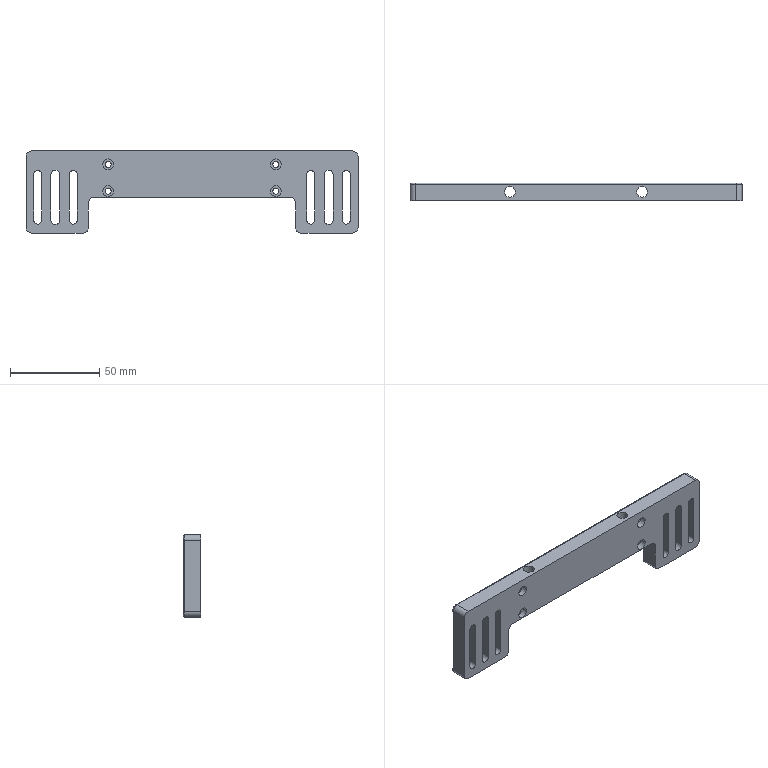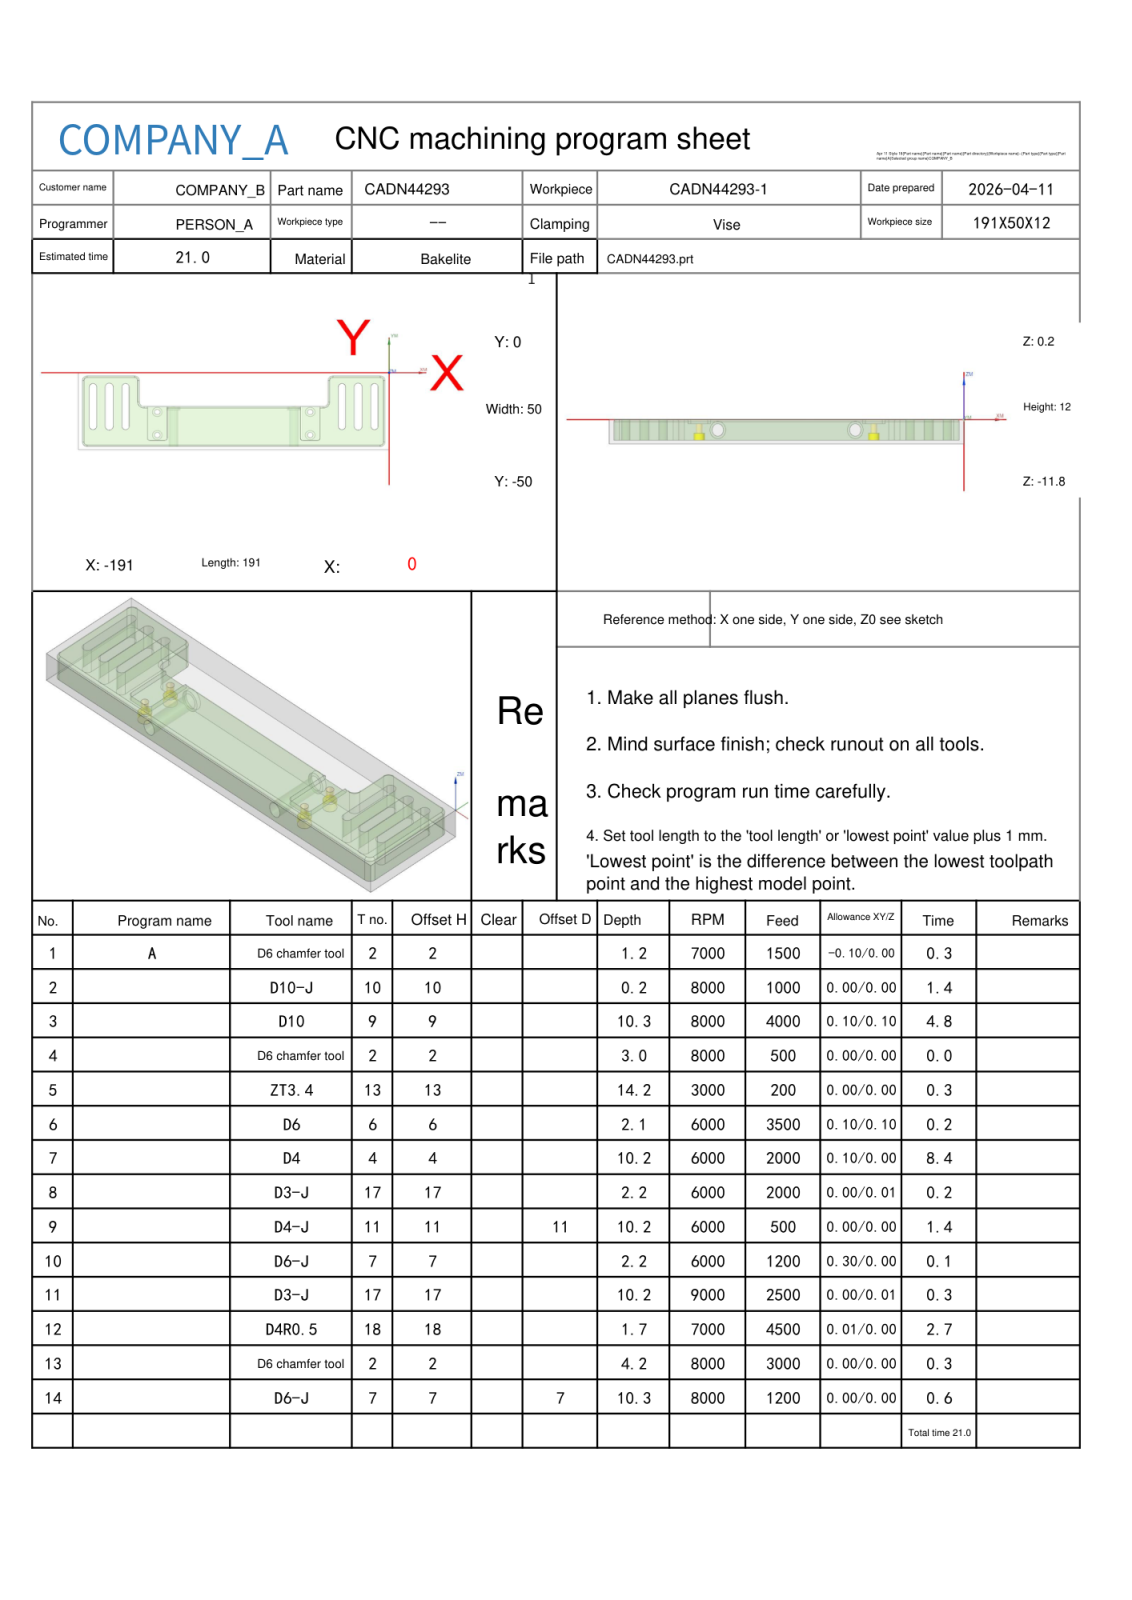NC program | NX | posted by the shop | part box 186 x 10 x 46 mm
Lines 4734 to 6466 of 7485, first 1444 of 1733 lines:
N11 T17 M06
(D3-J  D=3. R=0. H=17 ce=0.00 di=0.01)
G00 G90 G54 X-151.968 Y-16.863 M03 S9000
G43 H17 Z20.
M08
Z.474
G01 X-151.972 Y-16.864 Z.401 F2000.
X-151.984 Y-16.866 Z.328
X-152.001 Y-16.871 Z.256
X-152.024 Y-16.878 Z.185
X-152.051 Y-16.887 Z.115
X-152.081 Y-16.899 Z.049
X-152.112 Y-16.914 Z-.014
X-152.144 Y-16.932 Z-.073
X-152.176 Y-16.954 Z-.127
X-152.205 Y-16.978 Z-.174
X-152.232 Y-17.007 Z-.215
X-152.255 Y-17.04 Z-.247
X-152.273 Y-17.076 Z-.272
X-152.284 Y-17.117 Z-.287
X-152.288 Y-17.163 Z-.293
Y-19. F2500.
G03 X-150.5 Y-20.788 I1.788 J0.0
G01 X-148.663
X-148.634 Y-20.773 Z-.29
X-148.627 Y-20.729 Z-.283
X-148.642 Y-20.659 Z-.273
X-148.675 Y-20.567 Z-.26
X-148.726 Y-20.454 Z-.245
X-148.792 Y-20.324 Z-.23
X-148.964 Y-20.028 Z-.201
X-149.086 Y-19.835 Z-.186
X-149.298 Y-19.518 Z-.17
X-149.578 Y-19.138
X-149.88 Y-18.764 Z-.188
X-150.2 Y-18.401 Z-.223
X-150.535 Y-18.055 Z-.271
X-150.882 Y-17.731 Z-.331
X-151.178 Y-17.483 Z-.389
X-151.36 Y-17.341 Z-.426
X-151.641 Y-17.138 Z-.485
X-151.765 Y-17.059 Z-.512
X-151.873 Y-16.996 Z-.536
X-151.963 Y-16.954 Z-.557
X-152.03 Y-16.933 Z-.572
X-152.073 Y-16.935 Z-.582
X-152.088 Y-16.962 Z-.585
Y-19.
G03 X-150.5 Y-20.588 I1.588 J0.0
G01 X-148.55
X-148.521 Y-20.572 Z-.584
X-148.514 Y-20.527 Z-.582
X-148.529 Y-20.456 Z-.578
X-148.562 Y-20.361 Z-.574
X-148.612 Y-20.246 Z-.57
X-148.679 Y-20.115 Z-.565
X-148.85 Y-19.816 Z-.56
X-148.971 Y-19.622 Z-.558
X-149.183 Y-19.307 Z-.562
X-149.536 Y-18.844 Z-.583
X-149.923 Y-18.399 Z-.62
X-150.338 Y-17.98 Z-.668
X-150.774 Y-17.595 Z-.723
X-151.075 Y-17.363 Z-.761
X-151.261 Y-17.229 Z-.785
X-151.548 Y-17.04 Z-.821
X-151.675 Y-16.966 Z-.837
X-151.787 Y-16.909 Z-.85
X-151.878 Y-16.871 Z-.862
X-151.948 Y-16.852 Z-.871
X-151.992 Y-16.857 Z-.876
X-152.007 Y-16.885 Z-.878
Y-19.
G03 X-150.5 Y-20.507 I1.507 J0.0
G01 X-148.55
X-148.521 Y-20.491
X-148.514 Y-20.446 Z-.88
X-148.528 Y-20.374 Z-.882
X-148.561 Y-20.279 Z-.885
X-148.612 Y-20.164 Z-.889
X-148.678 Y-20.032 Z-.893
X-148.848 Y-19.734 Z-.906
X-148.969 Y-19.541 Z-.915
X-149.181 Y-19.228 Z-.932
X-149.532 Y-18.771 Z-.963
X-149.918 Y-18.336 Z-.999
X-150.332 Y-17.929 Z-1.038
X-150.768 Y-17.556 Z-1.077
X-151.068 Y-17.331 Z-1.102
X-151.254 Y-17.203 Z-1.116
X-151.541 Y-17.02 Z-1.138
X-151.669 Y-16.949 Z-1.147
X-151.78 Y-16.895 Z-1.155
X-151.871 Y-16.858 Z-1.162
X-151.941 Y-16.842 Z-1.167
X-151.985 Y-16.847 Z-1.17
X-152. Y-16.875 Z-1.171
Y-19.
G03 X-150.5 Y-20.5 I1.5 J0.0
G01 X-148.55
X-148.521 Y-20.484
X-148.514 Y-20.439 Z-1.174
X-148.528 Y-20.367 Z-1.178
X-148.561 Y-20.272 Z-1.184
X-148.612 Y-20.157 Z-1.19
X-148.678 Y-20.025 Z-1.198
X-148.848 Y-19.728 Z-1.217
X-148.969 Y-19.534 Z-1.229
X-149.181 Y-19.221 Z-1.25
X-149.532 Y-18.766 Z-1.283
X-149.918 Y-18.331 Z-1.317
X-150.332 Y-17.925 Z-1.351
X-150.768 Y-17.554 Z-1.384
X-151.068 Y-17.329 Z-1.405
X-151.254 Y-17.201 Z-1.417
X-151.541 Y-17.019 Z-1.436
X-151.669 Y-16.949 Z-1.443
X-151.78 Y-16.894 Z-1.45
X-151.871 Y-16.858 Z-1.456
X-151.941 Y-16.841 Z-1.46
X-151.985 Y-16.847 Z-1.462
X-152. Y-16.875 Z-1.463
Y-19.
G03 X-150.5 Y-20.5 I1.5 J0.0
G01 X-148.55
X-148.521 Y-20.484 Z-1.464
X-148.514 Y-20.439 Z-1.467
X-148.528 Y-20.367 Z-1.471
X-148.561 Y-20.272 Z-1.476
X-148.612 Y-20.157 Z-1.483
X-148.678 Y-20.025 Z-1.491
X-148.848 Y-19.728 Z-1.509
X-148.969 Y-19.534 Z-1.522
X-149.181 Y-19.221 Z-1.542
X-149.532 Y-18.766 Z-1.575
X-149.918 Y-18.331 Z-1.61
X-150.332 Y-17.925 Z-1.644
X-150.768 Y-17.554 Z-1.677
X-151.068 Y-17.329 Z-1.697
X-151.254 Y-17.201 Z-1.71
X-151.541 Y-17.019 Z-1.728
X-151.669 Y-16.949 Z-1.736
X-151.78 Y-16.894 Z-1.743
X-151.871 Y-16.858 Z-1.748
X-151.941 Y-16.841 Z-1.752
X-151.985 Y-16.846 Z-1.755
X-152. Y-16.875 Z-1.756
Y-19.
G03 X-150.5 Y-20.5 I1.5 J0.0
G01 X-148.55
X-148.521 Y-20.484 Z-1.757
X-148.514 Y-20.439 Z-1.759
X-148.528 Y-20.367 Z-1.763
X-148.561 Y-20.272 Z-1.769
X-148.612 Y-20.157 Z-1.776
X-148.678 Y-20.025 Z-1.784
X-148.848 Y-19.728 Z-1.802
X-148.969 Y-19.534 Z-1.814
X-149.181 Y-19.221 Z-1.835
X-149.532 Y-18.765 Z-1.868
X-149.918 Y-18.331 Z-1.902
X-150.332 Y-17.925 Z-1.936
X-150.768 Y-17.553 Z-1.969
X-151.068 Y-17.329 Z-1.99
X-151.254 Y-17.201 Z-2.002
X-151.541 Y-17.019 Z-2.021
X-151.669 Y-16.948 Z-2.029
X-151.78 Y-16.894 Z-2.035
X-151.871 Y-16.858 Z-2.041
X-151.941 Y-16.841 Z-2.045
X-151.985 Y-16.846 Z-2.048
X-152. Y-16.875 Z-2.049
Y-19.
G03 X-150.5 Y-20.5 I1.5 J0.0
G01 X-148.375
X-148.346 Y-20.484
X-148.341 Y-20.439 Z-2.052
X-148.357 Y-20.367 Z-2.056
X-148.394 Y-20.272 Z-2.062
X-148.448 Y-20.157 Z-2.068
X-148.519 Y-20.025 Z-2.076
X-148.7 Y-19.727 Z-2.095
X-148.829 Y-19.534 Z-2.107
X-149.053 Y-19.221 Z-2.128
X-149.424 Y-18.765 Z-2.161
X-149.83 Y-18.331 Z-2.195
X-150.265 Y-17.925 Z-2.229
X-150.72 Y-17.553 Z-2.262
X-151.034 Y-17.329 Z-2.283
X-151.227 Y-17.201 Z-2.295
X-151.525 Y-17.019 Z-2.313
X-151.657 Y-16.948 Z-2.321
X-151.772 Y-16.894 Z-2.328
X-151.867 Y-16.858 Z-2.334
X-151.939 Y-16.841 Z-2.338
X-151.984 Y-16.846 Z-2.34
X-152. Y-16.875 Z-2.341
Y-19.
G03 X-150.5 Y-20.5 I1.5 J0.0
G01 X-148.375
X-148.346 Y-20.484 Z-2.342
X-148.341 Y-20.439 Z-2.345
X-148.357 Y-20.367 Z-2.349
X-148.394 Y-20.272 Z-2.354
X-148.448 Y-20.157 Z-2.361
X-148.519 Y-20.025 Z-2.369
X-148.7 Y-19.727 Z-2.387
X-148.829 Y-19.534 Z-2.4
X-149.053 Y-19.221 Z-2.42
X-149.424 Y-18.765 Z-2.453
X-149.83 Y-18.331 Z-2.488
X-150.265 Y-17.925 Z-2.522
X-150.72 Y-17.553 Z-2.555
X-151.034 Y-17.329 Z-2.575
X-151.227 Y-17.201 Z-2.588
X-151.525 Y-17.019 Z-2.606
X-151.657 Y-16.948 Z-2.614
X-151.772 Y-16.894 Z-2.621
X-151.867 Y-16.858 Z-2.626
X-151.939 Y-16.841 Z-2.63
X-151.984 Y-16.846 Z-2.633
X-152. Y-16.875 Z-2.634
Y-19.
G03 X-150.5 Y-20.5 I1.5 J0.0
G01 X-148.375
X-148.346 Y-20.484 Z-2.635
X-148.341 Y-20.439 Z-2.637
X-148.357 Y-20.367 Z-2.641
X-148.394 Y-20.272 Z-2.647
X-148.448 Y-20.157 Z-2.654
X-148.519 Y-20.025 Z-2.662
X-148.7 Y-19.727 Z-2.68
X-148.829 Y-19.534 Z-2.692
X-149.053 Y-19.221 Z-2.713
X-149.424 Y-18.765 Z-2.746
X-149.83 Y-18.331 Z-2.78
X-150.265 Y-17.925 Z-2.814
X-150.72 Y-17.553 Z-2.847
X-151.034 Y-17.329 Z-2.868
X-151.227 Y-17.201 Z-2.88
X-151.525 Y-17.019 Z-2.899
X-151.657 Y-16.948 Z-2.907
X-151.772 Y-16.894 Z-2.913
X-151.867 Y-16.858 Z-2.919
X-151.939 Y-16.841 Z-2.923
X-151.984 Y-16.846 Z-2.926
X-152. Y-16.875
Y-19.
G03 X-150.5 Y-20.5 I1.5 J0.0
G01 X-148.375
X-148.346 Y-20.484 Z-2.927
X-148.341 Y-20.439 Z-2.93
X-148.357 Y-20.367 Z-2.934
X-148.394 Y-20.272 Z-2.94
X-148.448 Y-20.157 Z-2.946
X-148.519 Y-20.025 Z-2.954
X-148.7 Y-19.727 Z-2.973
X-148.829 Y-19.534 Z-2.985
X-149.053 Y-19.221 Z-3.006
X-149.424 Y-18.765 Z-3.039
X-149.83 Y-18.331 Z-3.073
X-150.265 Y-17.925 Z-3.107
X-150.72 Y-17.553 Z-3.14
X-151.034 Y-17.329 Z-3.161
X-151.227 Y-17.201 Z-3.173
X-151.525 Y-17.019 Z-3.191
X-151.657 Y-16.948 Z-3.199
X-151.772 Y-16.894 Z-3.206
X-151.867 Y-16.858 Z-3.212
X-151.939 Y-16.841 Z-3.216
X-151.984 Y-16.846 Z-3.218
X-152. Y-16.875 Z-3.219
Y-19.
G03 X-150.5 Y-20.5 I1.5 J0.0
G01 X-148.375
X-148.346 Y-20.484 Z-3.22
X-148.341 Y-20.439 Z-3.223
X-148.357 Y-20.367 Z-3.227
X-148.394 Y-20.272 Z-3.232
X-148.448 Y-20.157 Z-3.239
X-148.519 Y-20.025 Z-3.247
X-148.7 Y-19.727 Z-3.265
X-148.829 Y-19.534 Z-3.278
X-149.053 Y-19.221 Z-3.298
X-149.424 Y-18.765 Z-3.331
X-149.83 Y-18.331 Z-3.365
X-150.265 Y-17.925 Z-3.4
X-150.72 Y-17.553 Z-3.433
X-151.034 Y-17.329 Z-3.453
X-151.227 Y-17.201 Z-3.466
X-151.525 Y-17.019 Z-3.484
X-151.657 Y-16.948 Z-3.492
X-151.772 Y-16.894 Z-3.499
X-151.867 Y-16.858 Z-3.504
X-151.939 Y-16.841 Z-3.508
X-151.984 Y-16.846 Z-3.511
X-152. Y-16.875 Z-3.512
Y-19.
G03 X-150.5 Y-20.5 I1.5 J0.0
G01 X-148.375
X-148.346 Y-20.484 Z-3.513
X-148.341 Y-20.439 Z-3.515
X-148.357 Y-20.367 Z-3.519
X-148.394 Y-20.272 Z-3.525
X-148.448 Y-20.157 Z-3.532
X-148.519 Y-20.025 Z-3.539
X-148.7 Y-19.727 Z-3.558
X-148.829 Y-19.534 Z-3.57
X-149.053 Y-19.221 Z-3.591
X-149.424 Y-18.765 Z-3.624
X-149.83 Y-18.331 Z-3.658
X-150.265 Y-17.925 Z-3.692
X-150.72 Y-17.553 Z-3.725
X-151.034 Y-17.329 Z-3.746
X-151.227 Y-17.201 Z-3.758
X-151.525 Y-17.019 Z-3.777
X-151.657 Y-16.948 Z-3.785
X-151.772 Y-16.894 Z-3.791
X-151.867 Y-16.858 Z-3.797
X-151.939 Y-16.841 Z-3.801
X-151.984 Y-16.846 Z-3.804
X-152. Y-16.875
Y-19.
G03 X-150.5 Y-20.5 I1.5 J0.0
G01 X-148.375
X-148.346 Y-20.484 Z-3.805
X-148.341 Y-20.439 Z-3.808
X-148.357 Y-20.367 Z-3.812
X-148.394 Y-20.272 Z-3.817
X-148.448 Y-20.157 Z-3.824
X-148.519 Y-20.025 Z-3.832
X-148.7 Y-19.727 Z-3.85
X-148.829 Y-19.534 Z-3.863
X-149.053 Y-19.221 Z-3.884
X-149.424 Y-18.765 Z-3.917
X-149.83 Y-18.331 Z-3.951
X-150.265 Y-17.925 Z-3.985
X-150.72 Y-17.553 Z-4.018
X-151.034 Y-17.329 Z-4.039
X-151.227 Y-17.201 Z-4.051
X-151.525 Y-17.019 Z-4.069
X-151.657 Y-16.948 Z-4.077
X-151.772 Y-16.894 Z-4.084
X-151.867 Y-16.858 Z-4.09
X-151.939 Y-16.841 Z-4.094
X-151.984 Y-16.846 Z-4.096
X-152. Y-16.875 Z-4.097
Y-19.
G03 X-150.5 Y-20.5 I1.5 J0.0
G01 X-148.375
X-148.346 Y-20.484 Z-4.098
X-148.341 Y-20.439 Z-4.101
X-148.357 Y-20.367 Z-4.105
X-148.394 Y-20.272 Z-4.11
X-148.448 Y-20.157 Z-4.117
X-148.519 Y-20.025 Z-4.125
X-148.7 Y-19.727 Z-4.143
X-148.829 Y-19.534 Z-4.155
X-149.053 Y-19.221 Z-4.176
X-149.424 Y-18.765 Z-4.209
X-149.83 Y-18.331 Z-4.243
X-150.265 Y-17.925 Z-4.277
X-150.72 Y-17.553 Z-4.31
X-151.034 Y-17.329 Z-4.331
X-151.227 Y-17.201 Z-4.344
X-151.525 Y-17.019 Z-4.362
X-151.657 Y-16.948 Z-4.37
X-151.772 Y-16.894 Z-4.377
X-151.867 Y-16.858 Z-4.382
X-151.939 Y-16.841 Z-4.386
X-151.984 Y-16.846 Z-4.389
X-152. Y-16.875 Z-4.39
Y-19.
G03 X-150.5 Y-20.5 I1.5 J0.0
G01 X-148.375
X-148.346 Y-20.484 Z-4.391
X-148.341 Y-20.439 Z-4.393
X-148.357 Y-20.367 Z-4.397
X-148.394 Y-20.272 Z-4.403
X-148.448 Y-20.157 Z-4.41
X-148.519 Y-20.025 Z-4.417
X-148.7 Y-19.727 Z-4.436
X-148.829 Y-19.534 Z-4.448
X-149.053 Y-19.221 Z-4.469
X-149.424 Y-18.765 Z-4.502
X-149.83 Y-18.331 Z-4.536
X-150.265 Y-17.925 Z-4.57
X-150.72 Y-17.553 Z-4.603
X-151.034 Y-17.329 Z-4.624
X-151.227 Y-17.201 Z-4.636
X-151.525 Y-17.019 Z-4.655
X-151.657 Y-16.948 Z-4.663
X-151.772 Y-16.894 Z-4.669
X-151.867 Y-16.858 Z-4.675
X-151.939 Y-16.841 Z-4.679
X-151.984 Y-16.846 Z-4.681
X-152. Y-16.875 Z-4.682
Y-19.
G03 X-150.5 Y-20.5 I1.5 J0.0
G01 X-148.375
X-148.346 Y-20.484 Z-4.683
X-148.341 Y-20.439 Z-4.686
X-148.357 Y-20.367 Z-4.69
X-148.394 Y-20.272 Z-4.695
X-148.448 Y-20.157 Z-4.702
X-148.519 Y-20.025 Z-4.71
X-148.7 Y-19.727 Z-4.728
X-148.829 Y-19.534 Z-4.741
X-149.053 Y-19.221 Z-4.762
X-149.424 Y-18.765 Z-4.795
X-149.83 Y-18.331 Z-4.829
X-150.265 Y-17.925 Z-4.863
X-150.72 Y-17.553 Z-4.896
X-151.034 Y-17.329 Z-4.917
X-151.227 Y-17.201 Z-4.929
X-151.525 Y-17.019 Z-4.947
X-151.657 Y-16.948 Z-4.955
X-151.772 Y-16.894 Z-4.962
X-151.867 Y-16.858 Z-4.967
X-151.939 Y-16.841 Z-4.972
X-151.984 Y-16.846 Z-4.974
X-152. Y-16.875 Z-4.975
Y-19.
G03 X-150.5 Y-20.5 I1.5 J0.0
G01 X-148.375
X-148.346 Y-20.484 Z-4.976
X-148.341 Y-20.439 Z-4.978
X-148.357 Y-20.367 Z-4.983
X-148.394 Y-20.272 Z-4.988
X-148.448 Y-20.157 Z-4.995
X-148.519 Y-20.025 Z-5.003
X-148.7 Y-19.727 Z-5.021
X-148.829 Y-19.534 Z-5.033
X-149.053 Y-19.221 Z-5.054
X-149.424 Y-18.765 Z-5.087
X-149.83 Y-18.331 Z-5.121
X-150.265 Y-17.925 Z-5.155
X-150.72 Y-17.553 Z-5.188
X-151.034 Y-17.329 Z-5.209
X-151.227 Y-17.201 Z-5.222
X-151.525 Y-17.019 Z-5.24
X-151.657 Y-16.948 Z-5.248
X-151.772 Y-16.894 Z-5.255
X-151.867 Y-16.858 Z-5.26
X-151.939 Y-16.841 Z-5.264
X-151.984 Y-16.846 Z-5.267
X-152. Y-16.875 Z-5.268
Y-19.
G03 X-150.5 Y-20.5 I1.5 J0.0
G01 X-148.375
X-148.346 Y-20.484 Z-5.269
X-148.341 Y-20.439 Z-5.271
X-148.357 Y-20.367 Z-5.275
X-148.394 Y-20.272 Z-5.281
X-148.448 Y-20.157 Z-5.287
X-148.519 Y-20.025 Z-5.295
X-148.7 Y-19.727 Z-5.314
X-148.829 Y-19.534 Z-5.326
X-149.053 Y-19.221 Z-5.347
X-149.424 Y-18.765 Z-5.38
X-149.83 Y-18.331 Z-5.414
X-150.265 Y-17.925 Z-5.448
X-150.72 Y-17.553 Z-5.481
X-151.034 Y-17.329 Z-5.502
X-151.227 Y-17.201 Z-5.514
X-151.525 Y-17.019 Z-5.533
X-151.657 Y-16.948 Z-5.54
X-151.772 Y-16.894 Z-5.547
X-151.867 Y-16.858 Z-5.553
X-151.939 Y-16.841 Z-5.557
X-151.984 Y-16.846 Z-5.559
X-152. Y-16.875 Z-5.56
Y-19.
G03 X-150.5 Y-20.5 I1.5 J0.0
G01 X-148.375
X-148.346 Y-20.484 Z-5.561
X-148.341 Y-20.439 Z-5.564
X-148.357 Y-20.367 Z-5.568
X-148.394 Y-20.272 Z-5.573
X-148.448 Y-20.157 Z-5.58
X-148.519 Y-20.025 Z-5.588
X-148.7 Y-19.727 Z-5.606
X-148.829 Y-19.534 Z-5.619
X-149.053 Y-19.221 Z-5.64
X-149.424 Y-18.765 Z-5.673
X-149.83 Y-18.331 Z-5.707
X-150.265 Y-17.925 Z-5.741
X-150.72 Y-17.553 Z-5.774
X-151.034 Y-17.329 Z-5.795
X-151.227 Y-17.201 Z-5.807
X-151.525 Y-17.019 Z-5.825
X-151.657 Y-16.948 Z-5.833
X-151.772 Y-16.894 Z-5.84
X-151.867 Y-16.858 Z-5.845
X-151.939 Y-16.841 Z-5.849
X-151.984 Y-16.846 Z-5.852
X-152. Y-16.875 Z-5.853
Y-19.
G03 X-150.5 Y-20.5 I1.5 J0.0
G01 X-148.375
X-148.346 Y-20.484 Z-5.854
X-148.341 Y-20.439 Z-5.856
X-148.357 Y-20.367 Z-5.86
X-148.394 Y-20.272 Z-5.866
X-148.448 Y-20.157 Z-5.873
X-148.519 Y-20.025 Z-5.881
X-148.7 Y-19.727 Z-5.899
X-148.829 Y-19.534 Z-5.911
X-149.053 Y-19.221 Z-5.932
X-149.424 Y-18.765 Z-5.965
X-149.83 Y-18.331 Z-5.999
X-150.265 Y-17.925 Z-6.033
X-150.72 Y-17.553 Z-6.066
X-151.034 Y-17.329 Z-6.087
X-151.227 Y-17.201 Z-6.1
X-151.525 Y-17.019 Z-6.118
X-151.657 Y-16.948 Z-6.126
X-151.772 Y-16.894 Z-6.133
X-151.867 Y-16.858 Z-6.138
X-151.939 Y-16.841 Z-6.142
X-151.984 Y-16.846 Z-6.145
X-152. Y-16.875 Z-6.146
Y-19.
G03 X-150.5 Y-20.5 I1.5 J0.0
G01 X-148.375
X-148.346 Y-20.484
X-148.341 Y-20.439 Z-6.149
X-148.357 Y-20.367 Z-6.153
X-148.394 Y-20.272 Z-6.159
X-148.448 Y-20.157 Z-6.165
X-148.519 Y-20.025 Z-6.173
X-148.7 Y-19.727 Z-6.192
X-148.829 Y-19.534 Z-6.204
X-149.053 Y-19.221 Z-6.225
X-149.424 Y-18.765 Z-6.258
X-149.83 Y-18.331 Z-6.292
X-150.265 Y-17.925 Z-6.326
X-150.72 Y-17.553 Z-6.359
X-151.034 Y-17.329 Z-6.38
X-151.227 Y-17.201 Z-6.392
X-151.525 Y-17.019 Z-6.411
X-151.657 Y-16.948 Z-6.418
X-151.772 Y-16.894 Z-6.425
X-151.867 Y-16.858 Z-6.431
X-151.939 Y-16.841 Z-6.435
X-151.984 Y-16.846 Z-6.437
X-152. Y-16.875 Z-6.438
Y-19.
G03 X-150.5 Y-20.5 I1.5 J0.0
G01 X-148.375
X-148.346 Y-20.484 Z-6.439
X-148.341 Y-20.439 Z-6.442
X-148.357 Y-20.367 Z-6.446
X-148.394 Y-20.272 Z-6.451
X-148.448 Y-20.157 Z-6.458
X-148.519 Y-20.025 Z-6.466
X-148.7 Y-19.727 Z-6.484
X-148.829 Y-19.534 Z-6.497
X-149.053 Y-19.221 Z-6.517
X-149.424 Y-18.765 Z-6.55
X-149.83 Y-18.331 Z-6.585
X-150.265 Y-17.925 Z-6.619
X-150.72 Y-17.553 Z-6.652
X-151.034 Y-17.329 Z-6.672
X-151.227 Y-17.201 Z-6.685
X-151.525 Y-17.019 Z-6.703
X-151.657 Y-16.948 Z-6.711
X-151.772 Y-16.894 Z-6.718
X-151.867 Y-16.858 Z-6.723
X-151.939 Y-16.841 Z-6.727
X-151.984 Y-16.846 Z-6.73
X-152. Y-16.875 Z-6.731
Y-19.
G03 X-150.5 Y-20.5 I1.5 J0.0
G01 X-148.375
X-148.346 Y-20.484 Z-6.732
X-148.341 Y-20.439 Z-6.734
X-148.357 Y-20.367 Z-6.738
X-148.394 Y-20.272 Z-6.744
X-148.448 Y-20.157 Z-6.751
X-148.519 Y-20.025 Z-6.759
X-148.7 Y-19.727 Z-6.777
X-148.829 Y-19.534 Z-6.789
X-149.053 Y-19.221 Z-6.81
X-149.424 Y-18.765 Z-6.843
X-149.83 Y-18.331 Z-6.877
X-150.265 Y-17.925 Z-6.911
X-150.72 Y-17.553 Z-6.944
X-151.034 Y-17.329 Z-6.965
X-151.227 Y-17.201 Z-6.977
X-151.525 Y-17.019 Z-6.996
X-151.657 Y-16.948 Z-7.004
X-151.772 Y-16.894 Z-7.01
X-151.867 Y-16.858 Z-7.016
X-151.939 Y-16.841 Z-7.02
X-151.984 Y-16.846 Z-7.023
X-152. Y-16.875 Z-7.024
Y-19.
G03 X-150.5 Y-20.5 I1.5 J0.0
G01 X-148.375
X-148.346 Y-20.484
X-148.341 Y-20.439 Z-7.027
X-148.357 Y-20.367 Z-7.031
X-148.394 Y-20.272 Z-7.037
X-148.448 Y-20.157 Z-7.043
X-148.519 Y-20.025 Z-7.051
X-148.7 Y-19.727 Z-7.07
X-148.829 Y-19.534 Z-7.082
X-149.053 Y-19.221 Z-7.103
X-149.424 Y-18.765 Z-7.136
X-149.83 Y-18.331 Z-7.17
X-150.265 Y-17.925 Z-7.204
X-150.72 Y-17.553 Z-7.237
X-151.034 Y-17.329 Z-7.258
X-151.227 Y-17.201 Z-7.27
X-151.525 Y-17.019 Z-7.288
X-151.657 Y-16.948 Z-7.296
X-151.772 Y-16.894 Z-7.303
X-151.867 Y-16.858 Z-7.309
X-151.939 Y-16.841 Z-7.313
X-151.984 Y-16.846 Z-7.315
X-152. Y-16.875 Z-7.316
Y-19.
G03 X-150.5 Y-20.5 I1.5 J0.0
G01 X-148.375
X-148.346 Y-20.484 Z-7.317
X-148.341 Y-20.439 Z-7.32
X-148.357 Y-20.367 Z-7.324
X-148.394 Y-20.272 Z-7.329
X-148.448 Y-20.157 Z-7.336
X-148.519 Y-20.025 Z-7.344
X-148.7 Y-19.727 Z-7.362
X-148.829 Y-19.534 Z-7.375
X-149.053 Y-19.221 Z-7.395
X-149.424 Y-18.765 Z-7.428
X-149.83 Y-18.331 Z-7.463
X-150.265 Y-17.925 Z-7.497
X-150.72 Y-17.553 Z-7.53
X-151.034 Y-17.329 Z-7.55
X-151.227 Y-17.201 Z-7.563
X-151.525 Y-17.019 Z-7.581
X-151.657 Y-16.948 Z-7.589
X-151.772 Y-16.894 Z-7.596
X-151.867 Y-16.858 Z-7.601
X-151.939 Y-16.841 Z-7.605
X-151.984 Y-16.846 Z-7.608
X-152. Y-16.875 Z-7.609
Y-19.
G03 X-150.5 Y-20.5 I1.5 J0.0
G01 X-148.375
X-148.346 Y-20.484 Z-7.61
X-148.341 Y-20.439 Z-7.612
X-148.357 Y-20.367 Z-7.616
X-148.394 Y-20.272 Z-7.622
X-148.448 Y-20.157 Z-7.629
X-148.519 Y-20.025 Z-7.637
X-148.7 Y-19.727 Z-7.655
X-148.829 Y-19.534 Z-7.667
X-149.053 Y-19.221 Z-7.688
X-149.424 Y-18.765 Z-7.721
X-149.83 Y-18.331 Z-7.755
X-150.265 Y-17.925 Z-7.789
X-150.72 Y-17.553 Z-7.822
X-151.034 Y-17.329 Z-7.843
X-151.227 Y-17.201 Z-7.855
X-151.525 Y-17.019 Z-7.874
X-151.657 Y-16.948 Z-7.882
X-151.772 Y-16.894 Z-7.888
X-151.867 Y-16.858 Z-7.894
X-151.939 Y-16.841 Z-7.898
X-151.984 Y-16.846 Z-7.901
X-152. Y-16.875
Y-19.
G03 X-150.5 Y-20.5 I1.5 J0.0
G01 X-148.375
X-148.346 Y-20.484 Z-7.902
X-148.341 Y-20.439 Z-7.905
X-148.357 Y-20.367 Z-7.909
X-148.394 Y-20.272 Z-7.915
X-148.448 Y-20.157 Z-7.921
X-148.519 Y-20.025 Z-7.929
X-148.7 Y-19.727 Z-7.948
X-148.829 Y-19.534 Z-7.96
X-149.053 Y-19.221 Z-7.981
X-149.424 Y-18.765 Z-8.014
X-149.83 Y-18.331 Z-8.048
X-150.265 Y-17.925 Z-8.082
X-150.72 Y-17.553 Z-8.115
X-151.034 Y-17.329 Z-8.136
X-151.227 Y-17.201 Z-8.148
X-151.525 Y-17.019 Z-8.166
X-151.657 Y-16.948 Z-8.174
X-151.772 Y-16.894 Z-8.181
X-151.867 Y-16.858 Z-8.187
X-151.939 Y-16.841 Z-8.191
X-151.984 Y-16.846 Z-8.193
X-152. Y-16.875 Z-8.194
Y-19.
G03 X-150.5 Y-20.5 I1.5 J0.0
G01 X-148.375
X-148.346 Y-20.484 Z-8.195
X-148.341 Y-20.439 Z-8.198
X-148.357 Y-20.367 Z-8.202
X-148.394 Y-20.272 Z-8.207
X-148.448 Y-20.157 Z-8.214
X-148.519 Y-20.025 Z-8.222
X-148.7 Y-19.727 Z-8.24
X-148.829 Y-19.534 Z-8.253
X-149.053 Y-19.221 Z-8.273
X-149.424 Y-18.765 Z-8.306
X-149.83 Y-18.331 Z-8.34
X-150.265 Y-17.925 Z-8.375
X-150.72 Y-17.553 Z-8.408
X-151.034 Y-17.329 Z-8.428
X-151.227 Y-17.201 Z-8.441
X-151.525 Y-17.019 Z-8.459
X-151.657 Y-16.948 Z-8.467
X-151.772 Y-16.894 Z-8.474
X-151.867 Y-16.858 Z-8.479
X-151.939 Y-16.841 Z-8.483
X-151.984 Y-16.846 Z-8.486
X-152. Y-16.875 Z-8.487
Y-19.
G03 X-150.5 Y-20.5 I1.5 J0.0
G01 X-148.375
X-148.346 Y-20.484 Z-8.488
X-148.341 Y-20.439 Z-8.49
X-148.357 Y-20.367 Z-8.494
X-148.394 Y-20.272 Z-8.5
X-148.448 Y-20.157 Z-8.507
X-148.519 Y-20.025 Z-8.514
X-148.7 Y-19.727 Z-8.533
X-148.829 Y-19.534 Z-8.545
X-149.053 Y-19.221 Z-8.566
X-149.424 Y-18.765 Z-8.599
X-149.83 Y-18.331 Z-8.633
X-150.265 Y-17.925 Z-8.667
X-150.72 Y-17.553 Z-8.7
X-151.034 Y-17.329 Z-8.721
X-151.227 Y-17.201 Z-8.733
X-151.525 Y-17.019 Z-8.752
X-151.657 Y-16.948 Z-8.76
X-151.772 Y-16.894 Z-8.766
X-151.867 Y-16.858 Z-8.772
X-151.939 Y-16.841 Z-8.776
X-151.984 Y-16.846 Z-8.779
X-152. Y-16.875
Y-19.
G03 X-150.5 Y-20.5 I1.5 J0.0
G01 X-148.375
X-148.346 Y-20.484 Z-8.78
X-148.341 Y-20.439 Z-8.783
X-148.357 Y-20.367 Z-8.787
X-148.394 Y-20.272 Z-8.792
X-148.448 Y-20.157 Z-8.799
X-148.519 Y-20.025 Z-8.807
X-148.7 Y-19.727 Z-8.825
X-148.829 Y-19.534 Z-8.838
X-149.053 Y-19.221 Z-8.859
X-149.424 Y-18.765 Z-8.892
X-149.83 Y-18.331 Z-8.926
X-150.265 Y-17.925 Z-8.96
X-150.72 Y-17.553 Z-8.993
X-151.034 Y-17.329 Z-9.014
X-151.227 Y-17.201 Z-9.026
X-151.525 Y-17.019 Z-9.044
X-151.657 Y-16.948 Z-9.052
X-151.772 Y-16.894 Z-9.059
X-151.867 Y-16.858 Z-9.065
X-151.939 Y-16.841 Z-9.069
X-151.984 Y-16.846 Z-9.071
X-152. Y-16.875 Z-9.072
Y-19.
G03 X-150.5 Y-20.5 I1.5 J0.0
G01 X-148.375
X-148.346 Y-20.484 Z-9.073
X-148.341 Y-20.439 Z-9.076
X-148.357 Y-20.367 Z-9.08
X-148.394 Y-20.272 Z-9.085
X-148.448 Y-20.157 Z-9.092
X-148.519 Y-20.025 Z-9.1
X-148.7 Y-19.727 Z-9.118
X-148.829 Y-19.534 Z-9.13
X-149.053 Y-19.221 Z-9.151
X-149.424 Y-18.765 Z-9.184
X-149.83 Y-18.331 Z-9.218
X-150.265 Y-17.925 Z-9.252
X-150.72 Y-17.553 Z-9.285
X-151.034 Y-17.329 Z-9.306
X-151.227 Y-17.201 Z-9.319
X-151.525 Y-17.019 Z-9.337
X-151.657 Y-16.948 Z-9.345
X-151.772 Y-16.894 Z-9.352
X-151.867 Y-16.858 Z-9.357
X-151.939 Y-16.841 Z-9.361
X-151.984 Y-16.846 Z-9.364
X-152. Y-16.875 Z-9.365
Y-19.
G03 X-150.5 Y-20.5 I1.5 J0.0
G01 X-148.375
X-148.346 Y-20.484 Z-9.366
X-148.341 Y-20.439 Z-9.368
X-148.357 Y-20.367 Z-9.372
X-148.394 Y-20.272 Z-9.378
X-148.448 Y-20.157 Z-9.385
X-148.519 Y-20.025 Z-9.392
X-148.7 Y-19.727 Z-9.411
X-148.829 Y-19.534 Z-9.423
X-149.053 Y-19.221 Z-9.444
X-149.424 Y-18.765 Z-9.477
X-149.83 Y-18.331 Z-9.511
X-150.265 Y-17.925 Z-9.545
X-150.72 Y-17.553 Z-9.578
X-151.034 Y-17.329 Z-9.599
X-151.227 Y-17.201 Z-9.611
X-151.525 Y-17.019 Z-9.63
X-151.657 Y-16.948 Z-9.638
X-151.772 Y-16.894 Z-9.644
X-151.867 Y-16.858 Z-9.65
X-151.939 Y-16.841 Z-9.654
X-151.984 Y-16.846 Z-9.656
X-152. Y-16.875 Z-9.657
Y-19.
G03 X-150.5 Y-20.5 I1.5 J0.0
G01 X-148.375
X-148.346 Y-20.484 Z-9.658
X-148.341 Y-20.439 Z-9.661
X-148.357 Y-20.367 Z-9.665
X-148.394 Y-20.272 Z-9.67
X-148.448 Y-20.157 Z-9.677
X-148.519 Y-20.025 Z-9.685
X-148.7 Y-19.727 Z-9.703
X-148.829 Y-19.534 Z-9.716
X-149.053 Y-19.221 Z-9.737
X-149.424 Y-18.765 Z-9.77
X-149.83 Y-18.331 Z-9.804
X-150.265 Y-17.925 Z-9.838
X-150.72 Y-17.553 Z-9.871
X-151.034 Y-17.329 Z-9.892
X-151.227 Y-17.201 Z-9.904
X-151.525 Y-17.019 Z-9.922
X-151.657 Y-16.948 Z-9.93
X-151.772 Y-16.894 Z-9.937
X-151.867 Y-16.858 Z-9.942
X-151.939 Y-16.841 Z-9.947
X-151.984 Y-16.846 Z-9.949
X-152. Y-16.875 Z-9.95
Y-19.
G03 X-150.5 Y-20.5 I1.5 J0.0
G01 X-148.375
X-148.333 Y-20.475 Z-9.949
X-148.296 Y-20.441 Z-9.945
X-148.263 Y-20.401 Z-9.938
X-148.233 Y-20.355 Z-9.927
X-148.208 Y-20.305 Z-9.913
X-148.185 Y-20.253 Z-9.895
X-148.166 Y-20.2 Z-9.873
X-148.149 Y-20.147 Z-9.846
X-148.136 Y-20.097 Z-9.814
X-148.125 Y-20.05 Z-9.777
X-148.116 Y-20.009 Z-9.734
X-148.11 Y-19.973 Z-9.685
X-148.106 Y-19.947 Z-9.63
X-148.104 Y-19.929 Z-9.568
X-148.103 Y-19.923 Z-9.5
G00 Z3.
X-42.637 Y-20.469
Z.475
G01 Y-20.473 Z.402 F2000.
X-42.634 Y-20.485 Z.329
X-42.629 Y-20.502 Z.257
X-42.622 Y-20.525 Z.185
X-42.613 Y-20.552 Z.116
X-42.601 Y-20.581 Z.049
X-42.586 Y-20.613 Z-.014
X-42.568 Y-20.645 Z-.073
X-42.547 Y-20.676 Z-.126
X-42.522 Y-20.705 Z-.174
X-42.493 Y-20.732 Z-.214
X-42.461 Y-20.755 Z-.247
X-42.424 Y-20.773 Z-.272
X-42.383 Y-20.784 Z-.287
X-42.337 Y-20.788 Z-.293
X-40.5 F2500.
G03 X-38.712 Y-19. I0.0 J1.788
G01 Y-17.163
X-38.727 Y-17.134 Z-.29
X-38.77 Y-17.127 Z-.283
X-38.839 Y-17.142 Z-.273
X-38.93 Y-17.175 Z-.26
X-39.04 Y-17.226 Z-.246
X-39.168 Y-17.292 Z-.23
X-39.392 Y-17.422 Z-.207
X-39.649 Y-17.585 Z-.186
X-39.959 Y-17.798 Z-.17
X-40.332 Y-18.078
X-40.698 Y-18.38 Z-.189
X-41.053 Y-18.7 Z-.223
X-41.391 Y-19.035 Z-.272
X-41.707 Y-19.382 Z-.332
X-41.948 Y-19.678 Z-.389
X-42.086 Y-19.86 Z-.426
X-42.283 Y-20.141 Z-.485
X-42.36 Y-20.265 Z-.512
X-42.42 Y-20.373 Z-.536
X-42.461 Y-20.463 Z-.557
X-42.481 Y-20.53 Z-.572
X-42.478 Y-20.573 Z-.582
X-42.45 Y-20.588 Z-.585
X-40.5
G03 X-38.912 Y-19. I0.0 J1.588
G01 Y-16.962
X-38.927 Y-16.934 Z-.584
X-38.971 Y-16.928 Z-.582
X-39.04 Y-16.943 Z-.578
X-39.132 Y-16.978 Z-.574
X-39.243 Y-17.031 Z-.57
X-39.37 Y-17.1 Z-.565
X-39.593 Y-17.234 Z-.56
X-39.845 Y-17.401 Z-.558
X-40.149 Y-17.62 Z-.562
X-40.594 Y-17.983 Z-.583
X-41.02 Y-18.38 Z-.62
X-41.42 Y-18.805 Z-.668
X-41.786 Y-19.252 Z-.723
X-42.006 Y-19.559 Z-.761
X-42.133 Y-19.748 Z-.785
X-42.311 Y-20.04 Z-.821
X-42.38 Y-20.17 Z-.837
X-42.433 Y-20.283 Z-.85
X-42.469 Y-20.376 Z-.862
X-42.484 Y-20.447 Z-.871
X-42.479 Y-20.491 Z-.876
X-42.45 Y-20.507 Z-.878
X-40.5
G03 X-38.993 Y-19. I0.0 J1.507
G01 Y-16.885
X-39.008 Y-16.856
X-39.052 Y-16.851 Z-.879
X-39.122 Y-16.867 Z-.881
X-39.214 Y-16.903 Z-.884
X-39.325 Y-16.956 Z-.888
X-39.453 Y-17.026 Z-.892
X-39.675 Y-17.163 Z-.901
X-39.926 Y-17.334 Z-.912
X-40.227 Y-17.557 Z-.927
X-40.665 Y-17.927 Z-.957
X-41.081 Y-18.333 Z-.992
X-41.468 Y-18.766 Z-1.03
X-41.821 Y-19.222 Z-1.069
X-42.034 Y-19.535 Z-1.095
X-42.156 Y-19.728 Z-1.111
X-42.327 Y-20.025 Z-1.134
X-42.393 Y-20.157 Z-1.144
X-42.444 Y-20.272 Z-1.153
X-42.477 Y-20.367 Z-1.161
X-42.491 Y-20.439 Z-1.166
X-42.484 Y-20.484 Z-1.169
X-42.455 Y-20.5 Z-1.171
X-40.5
G03 X-39. Y-19. I0.0 J1.5
G01 Y-16.875
X-39.015 Y-16.847
X-39.059 Y-16.841 Z-1.174
X-39.129 Y-16.858 Z-1.178
X-39.22 Y-16.894 Z-1.183
X-39.332 Y-16.949 Z-1.19
X-39.459 Y-17.02 Z-1.197
X-39.746 Y-17.201 Z-1.215
X-39.932 Y-17.329 Z-1.227
X-40.233 Y-17.554 Z-1.247
X-40.67 Y-17.925 Z-1.279
X-41.085 Y-18.331 Z-1.312
X-41.471 Y-18.766 Z-1.346
X-41.823 Y-19.221 Z-1.379
X-42.036 Y-19.534 Z-1.401
X-42.157 Y-19.728 Z-1.414
X-42.327 Y-20.025 Z-1.433
X-42.393 Y-20.157 Z-1.442
X-42.444 Y-20.272 Z-1.449
X-42.477 Y-20.367 Z-1.455
X-42.491 Y-20.439 Z-1.459
X-42.484 Y-20.484 Z-1.462
X-42.455 Y-20.5 Z-1.463
X-40.5
G03 X-39. Y-19. I0.0 J1.5
G01 Y-16.875
X-39.015 Y-16.847 Z-1.464
X-39.059 Y-16.841 Z-1.467
X-39.129 Y-16.858 Z-1.471
X-39.22 Y-16.894 Z-1.476
X-39.332 Y-16.949 Z-1.483
X-39.459 Y-17.019 Z-1.49
X-39.746 Y-17.201 Z-1.509
X-39.932 Y-17.329 Z-1.521
X-40.233 Y-17.554 Z-1.541
X-40.67 Y-17.925 Z-1.574
X-41.084 Y-18.331 Z-1.607
X-41.471 Y-18.766 Z-1.641
X-41.823 Y-19.221 Z-1.674
X-42.035 Y-19.534 Z-1.696
X-42.157 Y-19.728 Z-1.708
X-42.327 Y-20.025 Z-1.727
X-42.393 Y-20.157 Z-1.735
X-42.444 Y-20.272 Z-1.742
X-42.477 Y-20.367 Z-1.748
X-42.491 Y-20.439 Z-1.752
X-42.484 Y-20.484 Z-1.755
X-42.455 Y-20.5 Z-1.756
X-40.5
G03 X-39. Y-19. I0.0 J1.5
G01 Y-16.875
X-39.016 Y-16.846 Z-1.757
X-39.061 Y-16.841 Z-1.759
X-39.133 Y-16.858 Z-1.763
X-39.228 Y-16.894 Z-1.769
X-39.343 Y-16.949 Z-1.776
X-39.475 Y-17.019 Z-1.784
X-39.773 Y-17.2 Z-1.802
X-39.966 Y-17.329 Z-1.814
X-40.279 Y-17.553 Z-1.835
X-40.735 Y-17.924 Z-1.868
X-41.169 Y-18.33 Z-1.902
X-41.575 Y-18.764 Z-1.936
X-41.947 Y-19.22 Z-1.969
X-42.171 Y-19.533 Z-1.99
X-42.299 Y-19.727 Z-2.002
X-42.481 Y-20.024 Z-2.021
X-42.552 Y-20.157 Z-2.029
X-42.606 Y-20.272 Z-2.035
X-42.642 Y-20.367 Z-2.041
X-42.659 Y-20.439 Z-2.045
X-42.654 Y-20.484 Z-2.048
X-42.625 Y-20.5 Z-2.049
X-40.5
G03 X-39. Y-19. I0.0 J1.5
G01 Y-16.875
X-39.016 Y-16.846
X-39.061 Y-16.841 Z-2.052
X-39.133 Y-16.857 Z-2.056
X-39.228 Y-16.894 Z-2.062
X-39.343 Y-16.948 Z-2.068
X-39.475 Y-17.019 Z-2.076
X-39.773 Y-17.2 Z-2.095
X-39.966 Y-17.329 Z-2.107
X-40.279 Y-17.553 Z-2.128
X-40.735 Y-17.924 Z-2.161
X-41.169 Y-18.33 Z-2.195
X-41.575 Y-18.764 Z-2.229
X-41.947 Y-19.22 Z-2.262
X-42.171 Y-19.533 Z-2.283
X-42.299 Y-19.727 Z-2.295
X-42.481 Y-20.024 Z-2.313
X-42.552 Y-20.157 Z-2.321
X-42.606 Y-20.272 Z-2.328
X-42.642 Y-20.367 Z-2.334
X-42.659 Y-20.439 Z-2.338
X-42.654 Y-20.484 Z-2.34
X-42.625 Y-20.5 Z-2.341
X-40.5
G03 X-39. Y-19. I0.0 J1.5
G01 Y-16.875
X-39.016 Y-16.846 Z-2.342
X-39.061 Y-16.841 Z-2.345
X-39.133 Y-16.857 Z-2.349
X-39.228 Y-16.894 Z-2.354
X-39.343 Y-16.948 Z-2.361
X-39.475 Y-17.019 Z-2.369
X-39.773 Y-17.2 Z-2.387
X-39.966 Y-17.329 Z-2.4
X-40.279 Y-17.553 Z-2.42
X-40.735 Y-17.924 Z-2.453
X-41.169 Y-18.33 Z-2.487
X-41.575 Y-18.764 Z-2.522
X-41.947 Y-19.22 Z-2.555
X-42.171 Y-19.533 Z-2.575
X-42.299 Y-19.727 Z-2.588
X-42.481 Y-20.024 Z-2.606
X-42.552 Y-20.157 Z-2.614
X-42.606 Y-20.272 Z-2.621
X-42.642 Y-20.367 Z-2.626
X-42.659 Y-20.439 Z-2.63
X-42.654 Y-20.484 Z-2.633
X-42.625 Y-20.5 Z-2.634
X-40.5
G03 X-39. Y-19. I0.0 J1.5
G01 Y-16.875
X-39.016 Y-16.846 Z-2.635
X-39.061 Y-16.841 Z-2.637
X-39.133 Y-16.857 Z-2.641
X-39.228 Y-16.894 Z-2.647
X-39.343 Y-16.948 Z-2.654
X-39.475 Y-17.019 Z-2.662
X-39.773 Y-17.2 Z-2.68
X-39.966 Y-17.329 Z-2.692
X-40.279 Y-17.553 Z-2.713
X-40.735 Y-17.924 Z-2.746
X-41.169 Y-18.33 Z-2.78
X-41.575 Y-18.764 Z-2.814
X-41.947 Y-19.22 Z-2.847
X-42.171 Y-19.533 Z-2.868
X-42.299 Y-19.727 Z-2.88
X-42.481 Y-20.024 Z-2.899
X-42.552 Y-20.157 Z-2.907
X-42.606 Y-20.272 Z-2.913
X-42.642 Y-20.367 Z-2.919
X-42.659 Y-20.439 Z-2.923
X-42.654 Y-20.484 Z-2.926
X-42.625 Y-20.5
X-40.5
G03 X-39. Y-19. I0.0 J1.5
G01 Y-16.875
X-39.016 Y-16.846 Z-2.927
X-39.061 Y-16.841 Z-2.93
X-39.133 Y-16.857 Z-2.934
X-39.228 Y-16.894 Z-2.94
X-39.343 Y-16.948 Z-2.946
X-39.475 Y-17.019 Z-2.954
X-39.773 Y-17.2 Z-2.973
X-39.966 Y-17.329 Z-2.985
X-40.279 Y-17.553 Z-3.006
X-40.735 Y-17.924 Z-3.039
X-41.169 Y-18.33 Z-3.073
X-41.575 Y-18.764 Z-3.107
X-41.947 Y-19.22 Z-3.14
X-42.171 Y-19.533 Z-3.161
X-42.299 Y-19.727 Z-3.173
X-42.481 Y-20.025 Z-3.191
X-42.552 Y-20.157 Z-3.199
X-42.606 Y-20.272 Z-3.206
X-42.642 Y-20.367 Z-3.212
X-42.659 Y-20.439 Z-3.216
X-42.654 Y-20.484 Z-3.218
X-42.625 Y-20.5 Z-3.219
X-40.5
G03 X-39. Y-19. I0.0 J1.5
G01 Y-16.875
X-39.016 Y-16.846 Z-3.22
X-39.061 Y-16.841 Z-3.223
X-39.133 Y-16.857 Z-3.227
X-39.228 Y-16.894 Z-3.232
X-39.343 Y-16.948 Z-3.239
X-39.475 Y-17.019 Z-3.247
X-39.773 Y-17.2 Z-3.265
X-39.966 Y-17.329 Z-3.278
X-40.279 Y-17.553 Z-3.298
X-40.735 Y-17.924 Z-3.331
X-41.169 Y-18.33 Z-3.365
X-41.575 Y-18.764 Z-3.4
X-41.947 Y-19.22 Z-3.432
X-42.171 Y-19.533 Z-3.453
X-42.299 Y-19.727 Z-3.466
X-42.481 Y-20.025 Z-3.484
X-42.552 Y-20.157 Z-3.492
X-42.606 Y-20.272 Z-3.499
X-42.642 Y-20.367 Z-3.504
X-42.659 Y-20.439 Z-3.508
X-42.654 Y-20.484 Z-3.511
X-42.625 Y-20.5 Z-3.512
X-40.5
G03 X-39. Y-19. I0.0 J1.5
G01 Y-16.875
X-39.016 Y-16.846 Z-3.513
X-39.061 Y-16.841 Z-3.515
X-39.133 Y-16.857 Z-3.519
X-39.228 Y-16.894 Z-3.525
X-39.343 Y-16.948 Z-3.532
X-39.475 Y-17.019 Z-3.539
X-39.773 Y-17.2 Z-3.558
X-39.966 Y-17.329 Z-3.57
X-40.279 Y-17.553 Z-3.591
X-40.735 Y-17.924 Z-3.624
X-41.169 Y-18.33 Z-3.658
X-41.575 Y-18.765 Z-3.692
X-41.947 Y-19.22 Z-3.725
X-42.171 Y-19.534 Z-3.746
X-42.299 Y-19.727 Z-3.758
X-42.481 Y-20.025 Z-3.777
X-42.552 Y-20.157 Z-3.785
X-42.606 Y-20.272 Z-3.791
X-42.642 Y-20.367 Z-3.797
X-42.659 Y-20.439 Z-3.801
X-42.654 Y-20.484 Z-3.804
X-42.625 Y-20.5
X-40.5
G03 X-39. Y-19. I0.0 J1.5
G01 Y-16.875
X-39.016 Y-16.846 Z-3.805
X-39.061 Y-16.841 Z-3.808
X-39.133 Y-16.857 Z-3.812
X-39.228 Y-16.894 Z-3.817
X-39.343 Y-16.948 Z-3.824
X-39.475 Y-17.019 Z-3.832
X-39.773 Y-17.2 Z-3.85
X-39.966 Y-17.329 Z-3.863
X-40.279 Y-17.553 Z-3.884
X-40.735 Y-17.924 Z-3.917
X-41.169 Y-18.33 Z-3.951
X-41.575 Y-18.765 Z-3.985
X-41.947 Y-19.22 Z-4.018
X-42.171 Y-19.534 Z-4.039
X-42.299 Y-19.727 Z-4.051
X-42.481 Y-20.025 Z-4.069
X-42.552 Y-20.157 Z-4.077
X-42.606 Y-20.272 Z-4.084
X-42.642 Y-20.367 Z-4.09
X-42.659 Y-20.439 Z-4.094
X-42.654 Y-20.484 Z-4.096
X-42.625 Y-20.5 Z-4.097
X-40.5
G03 X-39. Y-19. I0.0 J1.5
G01 Y-16.875
X-39.016 Y-16.846 Z-4.098
X-39.061 Y-16.841 Z-4.101
X-39.133 Y-16.857 Z-4.105
X-39.228 Y-16.894 Z-4.11
X-39.343 Y-16.948 Z-4.117
X-39.475 Y-17.019 Z-4.125
X-39.773 Y-17.2 Z-4.143
X-39.966 Y-17.329 Z-4.155
X-40.279 Y-17.553 Z-4.176
X-40.735 Y-17.924 Z-4.209
X-41.169 Y-18.33 Z-4.243
X-41.575 Y-18.765 Z-4.277
X-41.947 Y-19.221 Z-4.31
X-42.171 Y-19.534 Z-4.331
X-42.299 Y-19.727 Z-4.344
X-42.481 Y-20.025 Z-4.362
X-42.552 Y-20.157 Z-4.37
X-42.606 Y-20.272 Z-4.377
X-42.642 Y-20.367 Z-4.382
X-42.659 Y-20.439 Z-4.386
X-42.654 Y-20.484 Z-4.389
X-42.625 Y-20.5 Z-4.39
X-40.5
G03 X-39. Y-19. I0.0 J1.5
G01 Y-16.875
X-39.016 Y-16.846 Z-4.391
X-39.061 Y-16.841 Z-4.393
X-39.133 Y-16.858 Z-4.397
X-39.228 Y-16.894 Z-4.403
X-39.343 Y-16.948 Z-4.41
X-39.475 Y-17.019 Z-4.417
X-39.773 Y-17.2 Z-4.436
X-39.966 Y-17.329 Z-4.448
X-40.279 Y-17.553 Z-4.469
X-40.735 Y-17.924 Z-4.502
X-41.169 Y-18.33 Z-4.536
X-41.575 Y-18.765 Z-4.57
X-41.947 Y-19.221 Z-4.603
X-42.171 Y-19.534 Z-4.624
X-42.299 Y-19.727 Z-4.636
X-42.481 Y-20.025 Z-4.655
X-42.552 Y-20.157 Z-4.663
X-42.606 Y-20.272 Z-4.669
X-42.642 Y-20.367 Z-4.675
X-42.659 Y-20.439 Z-4.679
X-42.654 Y-20.484 Z-4.681
X-42.625 Y-20.5 Z-4.682
X-40.5
G03 X-39. Y-19. I0.0 J1.5
G01 Y-16.875
X-39.016 Y-16.846 Z-4.683
X-39.061 Y-16.841 Z-4.686
X-39.133 Y-16.858 Z-4.69
X-39.228 Y-16.894 Z-4.695
X-39.343 Y-16.948 Z-4.702
X-39.475 Y-17.019 Z-4.71
X-39.773 Y-17.2 Z-4.728
X-39.966 Y-17.329 Z-4.741
X-40.279 Y-17.553 Z-4.762
X-40.735 Y-17.924 Z-4.795
X-41.169 Y-18.33 Z-4.829
X-41.575 Y-18.765 Z-4.863
X-41.947 Y-19.221 Z-4.896
X-42.171 Y-19.534 Z-4.917
X-42.299 Y-19.727 Z-4.929
X-42.481 Y-20.025 Z-4.947
X-42.552 Y-20.157 Z-4.955
X-42.606 Y-20.272 Z-4.962
X-42.642 Y-20.367 Z-4.967
X-42.659 Y-20.439 Z-4.972
X-42.654 Y-20.484 Z-4.974
X-42.625 Y-20.5 Z-4.975
X-40.5
G03 X-39. Y-19. I0.0 J1.5
G01 Y-16.875
X-39.016 Y-16.846 Z-4.976
X-39.061 Y-16.841 Z-4.978
X-39.133 Y-16.858 Z-4.983
X-39.228 Y-16.894 Z-4.988
X-39.343 Y-16.948 Z-4.995
X-39.475 Y-17.019 Z-5.003
X-39.773 Y-17.2 Z-5.021
X-39.966 Y-17.329 Z-5.033
X-40.279 Y-17.553 Z-5.054
X-40.735 Y-17.924 Z-5.087
X-41.169 Y-18.331 Z-5.121
X-41.575 Y-18.765 Z-5.155
X-41.947 Y-19.221 Z-5.188
X-42.171 Y-19.534 Z-5.209
X-42.299 Y-19.727 Z-5.222
X-42.481 Y-20.025 Z-5.24
X-42.552 Y-20.157 Z-5.248
X-42.606 Y-20.272 Z-5.255
X-42.642 Y-20.367 Z-5.26
X-42.659 Y-20.439 Z-5.264
X-42.654 Y-20.484 Z-5.267
X-42.625 Y-20.5 Z-5.268
X-40.5
G03 X-39. Y-19. I0.0 J1.5
G01 Y-16.875
X-39.016 Y-16.846 Z-5.269
X-39.061 Y-16.841 Z-5.271
X-39.133 Y-16.858 Z-5.275
X-39.228 Y-16.894 Z-5.281
X-39.343 Y-16.948 Z-5.287
X-39.475 Y-17.019 Z-5.295
X-39.773 Y-17.2 Z-5.314
X-39.966 Y-17.329 Z-5.326
X-40.279 Y-17.553 Z-5.347
X-40.735 Y-17.924 Z-5.38
X-41.169 Y-18.331 Z-5.414
X-41.575 Y-18.765 Z-5.448
X-41.947 Y-19.221 Z-5.481
X-42.171 Y-19.534 Z-5.502
X-42.299 Y-19.727 Z-5.514
X-42.481 Y-20.025 Z-5.533
X-42.552 Y-20.157 Z-5.54
X-42.606 Y-20.272 Z-5.547
X-42.642 Y-20.367 Z-5.553
X-42.659 Y-20.439 Z-5.557
X-42.654 Y-20.484 Z-5.559
X-42.625 Y-20.5 Z-5.56
X-40.5
G03 X-39. Y-19. I0.0 J1.5
G01 Y-16.875
X-39.016 Y-16.846 Z-5.561
X-39.061 Y-16.841 Z-5.564
X-39.133 Y-16.858 Z-5.568
X-39.228 Y-16.894 Z-5.573
X-39.343 Y-16.948 Z-5.58
X-39.475 Y-17.019 Z-5.588
X-39.773 Y-17.2 Z-5.606
X-39.966 Y-17.329 Z-5.619
X-40.279 Y-17.553 Z-5.64
X-40.735 Y-17.925 Z-5.673
X-41.169 Y-18.331 Z-5.707
X-41.575 Y-18.765 Z-5.741
X-41.947 Y-19.221 Z-5.774
X-42.171 Y-19.534 Z-5.794
X-42.299 Y-19.727 Z-5.807
X-42.481 Y-20.025 Z-5.825
X-42.552 Y-20.157 Z-5.833
X-42.606 Y-20.272 Z-5.84
X-42.642 Y-20.367 Z-5.845
X-42.659 Y-20.439 Z-5.849
X-42.654 Y-20.484 Z-5.852
X-42.625 Y-20.5 Z-5.853
X-40.5
G03 X-39. Y-19. I0.0 J1.5
G01 Y-16.875
X-39.016 Y-16.846 Z-5.854
X-39.061 Y-16.841 Z-5.856
X-39.133 Y-16.858 Z-5.86
X-39.228 Y-16.894 Z-5.866
X-39.343 Y-16.948 Z-5.873
X-39.475 Y-17.019 Z-5.881
X-39.773 Y-17.2 Z-5.899
X-39.966 Y-17.329 Z-5.911
X-40.279 Y-17.553 Z-5.932
X-40.735 Y-17.925 Z-5.965
X-41.169 Y-18.331 Z-5.999
X-41.575 Y-18.765 Z-6.033
X-41.947 Y-19.221 Z-6.066
X-42.171 Y-19.534 Z-6.087
X-42.299 Y-19.727 Z-6.099
X-42.481 Y-20.025 Z-6.118
X-42.552 Y-20.157 Z-6.126
X-42.606 Y-20.272 Z-6.133
X-42.642 Y-20.367 Z-6.138
X-42.659 Y-20.439 Z-6.142
X-42.654 Y-20.484 Z-6.145
X-42.625 Y-20.5 Z-6.146
X-40.5
G03 X-39. Y-19. I0.0 J1.5
G01 Y-16.875
X-39.016 Y-16.846
X-39.061 Y-16.841 Z-6.149
X-39.133 Y-16.858 Z-6.153
X-39.228 Y-16.894 Z-6.159
X-39.343 Y-16.948 Z-6.165
X-39.475 Y-17.019 Z-6.173
X-39.773 Y-17.2 Z-6.192
X-39.966 Y-17.329 Z-6.204
X-40.279 Y-17.553 Z-6.225
X-40.735 Y-17.925 Z-6.258
X-41.169 Y-18.331 Z-6.292
X-41.575 Y-18.765 Z-6.326
X-41.947 Y-19.221 Z-6.359
X-42.171 Y-19.534 Z-6.38
X-42.299 Y-19.727 Z-6.392
X-42.481 Y-20.025 Z-6.411
X-42.552 Y-20.157 Z-6.418
X-42.606 Y-20.272 Z-6.425
X-42.642 Y-20.367 Z-6.431
X-42.659 Y-20.439 Z-6.435
X-42.654 Y-20.484 Z-6.437
X-42.625 Y-20.5 Z-6.438
X-40.5
G03 X-39. Y-19. I0.0 J1.5
G01 Y-16.875
X-39.016 Y-16.846 Z-6.439
X-39.061 Y-16.841 Z-6.442
X-39.133 Y-16.858 Z-6.446
X-39.228 Y-16.894 Z-6.451
X-39.343 Y-16.948 Z-6.458
X-39.475 Y-17.019 Z-6.466
X-39.773 Y-17.2 Z-6.484
X-39.966 Y-17.329 Z-6.497
X-40.279 Y-17.553 Z-6.517
X-40.735 Y-17.925 Z-6.55
X-41.169 Y-18.331 Z-6.585
X-41.575 Y-18.765 Z-6.619
X-41.947 Y-19.221 Z-6.652
X-42.171 Y-19.534 Z-6.672
X-42.299 Y-19.727 Z-6.685
X-42.481 Y-20.025 Z-6.703
X-42.552 Y-20.157 Z-6.711
X-42.606 Y-20.272 Z-6.718
X-42.642 Y-20.367 Z-6.723
X-42.659 Y-20.439 Z-6.727
X-42.654 Y-20.484 Z-6.73
X-42.625 Y-20.5 Z-6.731
X-40.5
G03 X-39. Y-19. I0.0 J1.5
G01 Y-16.875
X-39.016 Y-16.846 Z-6.732
X-39.061 Y-16.841 Z-6.734
X-39.133 Y-16.858 Z-6.738
X-39.228 Y-16.894 Z-6.744
X-39.343 Y-16.948 Z-6.751
X-39.475 Y-17.019 Z-6.759
X-39.773 Y-17.2 Z-6.777